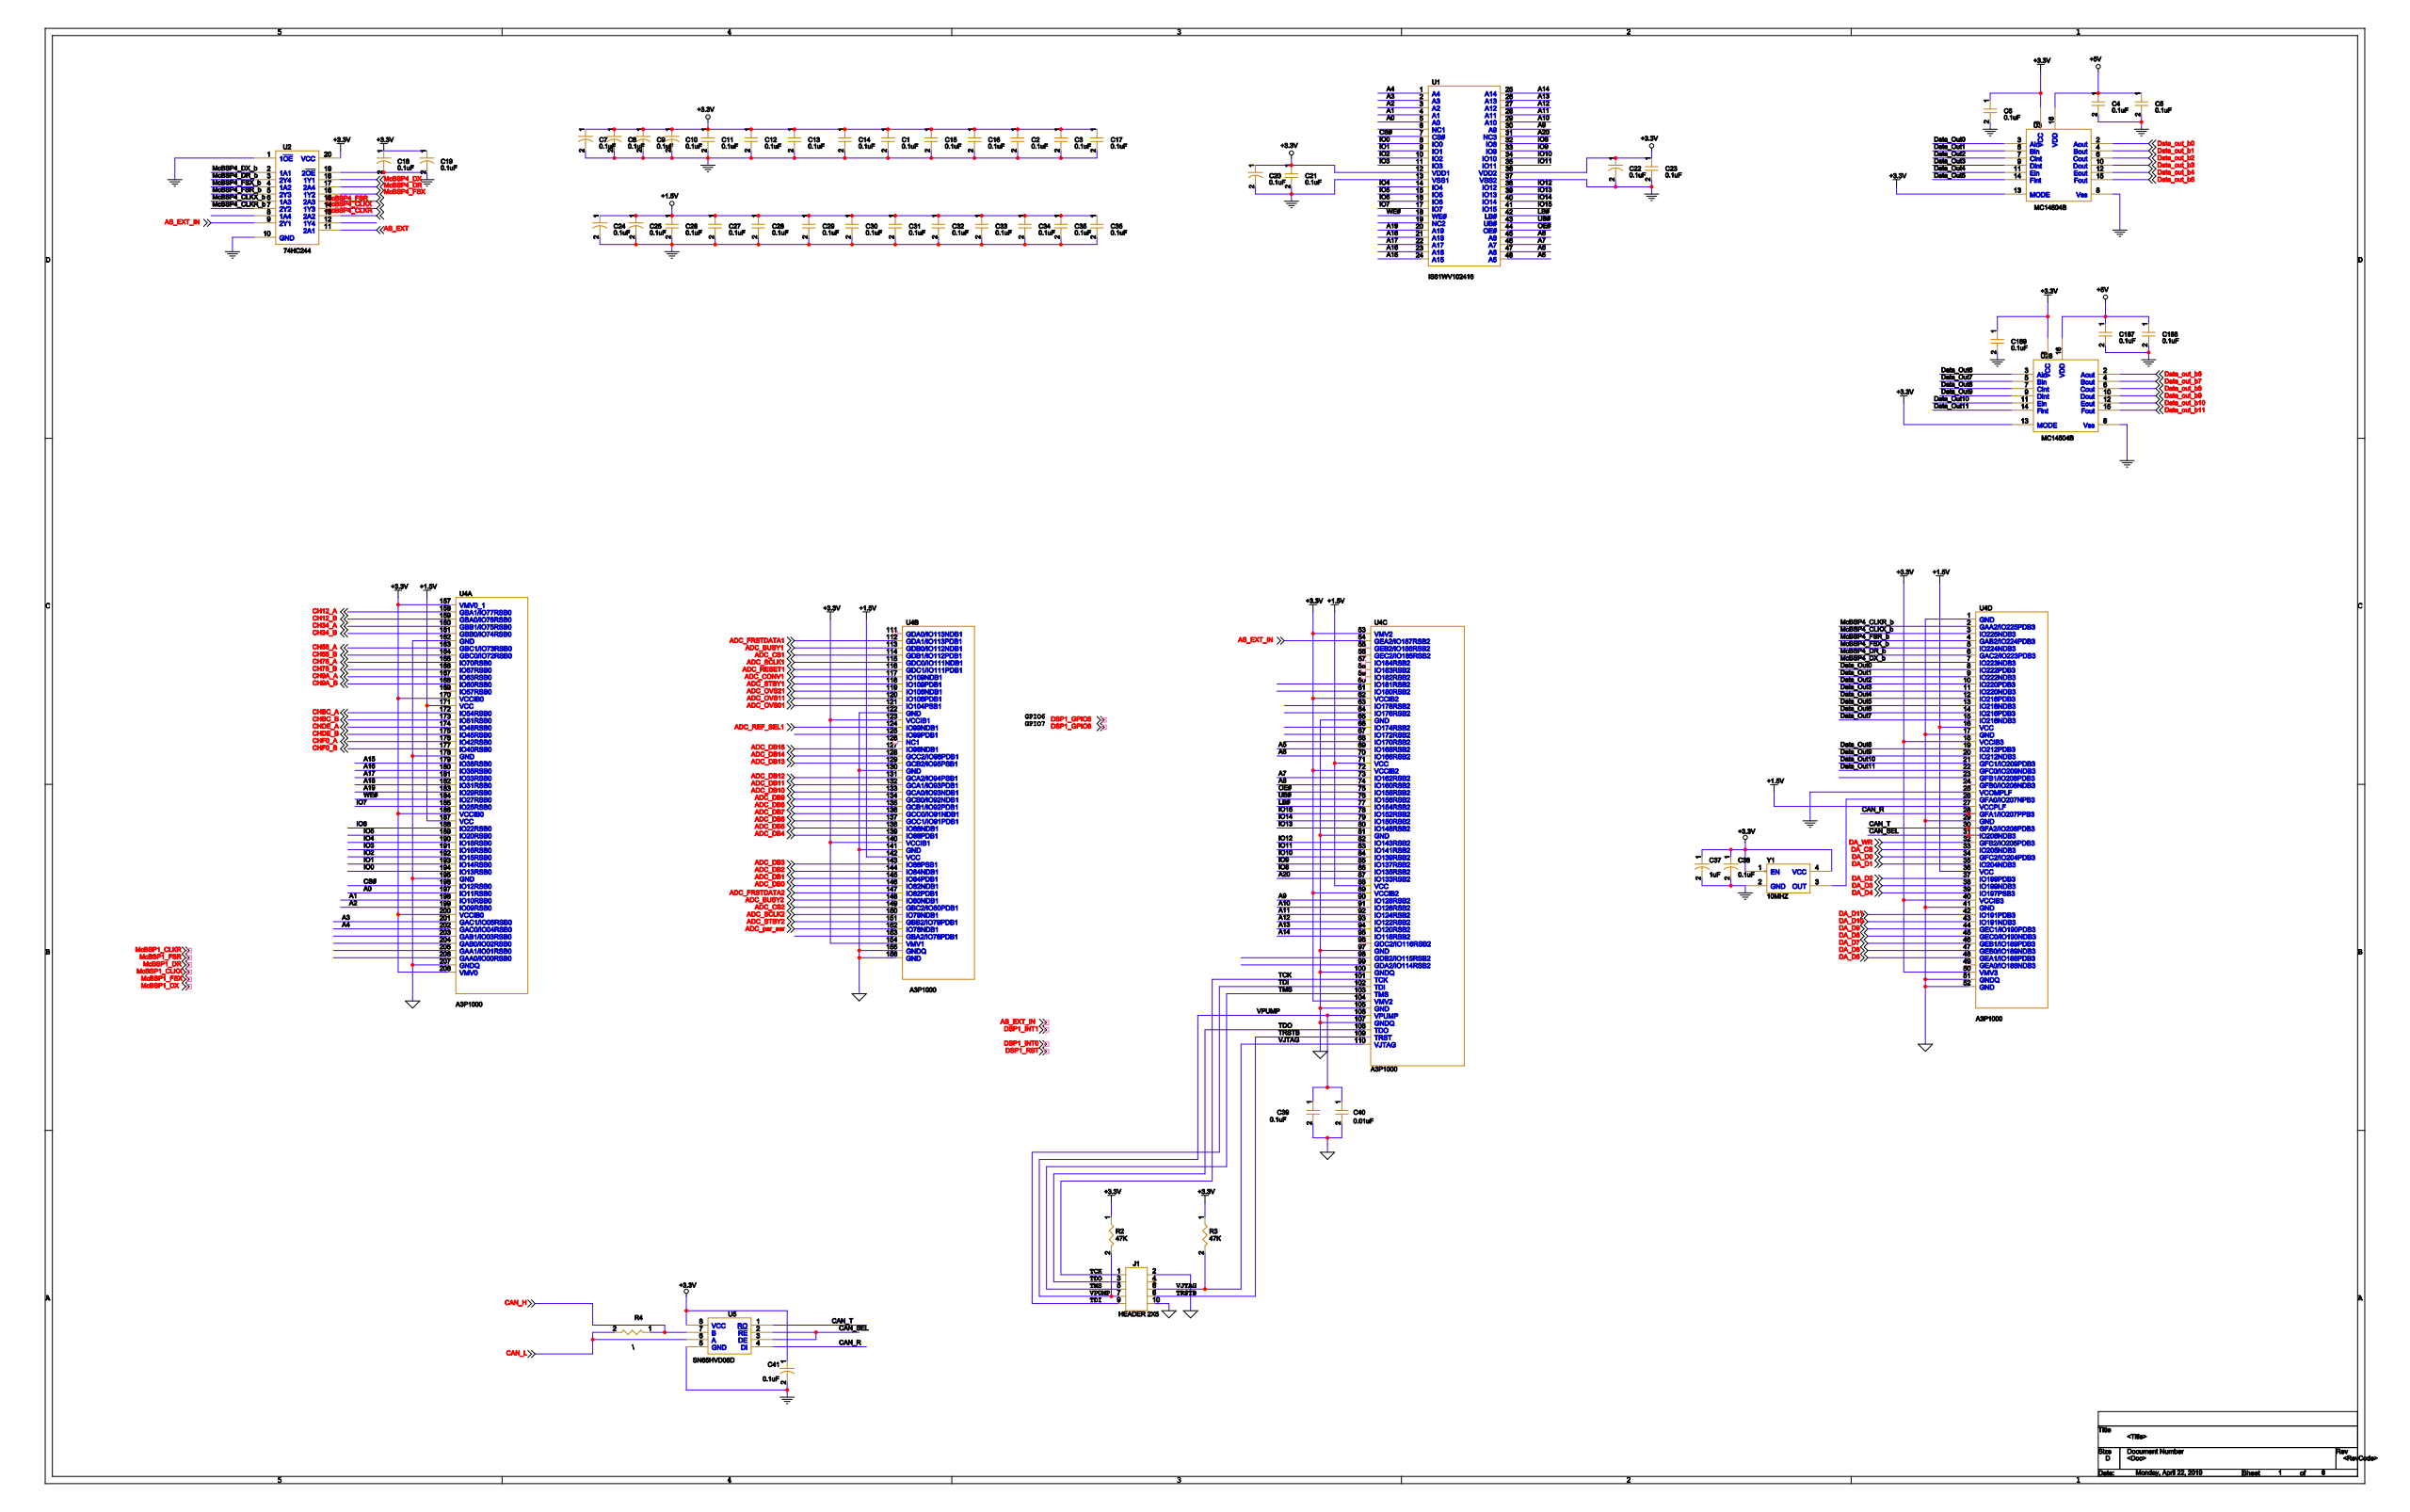Circuit board | Cadence Allegro | 362 parts | 391 nets | one sheet of the schematic
Parts on this sheet (reference | value | footprint):
C1 | 0.1uF | 1206
C2 | 0.1uF | 1206
C3 | 0.1uF | 1206
C4 | 0.1uF | 1206
C5 | 0.1uF | 1206
C6 | 0.1uF | 1206
C7 | 0.1uF | 1206
C8 | 0.1uF | 1206
C9 | 0.1uF | 1206
C10 | 0.1uF | 1206
C11 | 0.1uF | 1206
C12 | 0.1uF | 1206
C13 | 0.1uF | 1206
C14 | 0.1uF | 1206
C15 | 0.1uF | 1206
C16 | 0.1uF | 1206
C17 | 0.1uF | 1206
C18 | 0.1uF | 1206
C19 | 0.1uF | 1206
C20 | 0.1uF | 1206
C21 | 0.1uF | 1206
C22 | 0.1uF | 1206
C23 | 0.1uF | 1206
C24 | 0.1uF | 1206
C25 | 0.1uF | 1206
C26 | 0.1uF | 1206
C27 | 0.1uF | 1206
C28 | 0.1uF | 1206
C29 | 0.1uF | 1206
C30 | 0.1uF | 1206
C31 | 0.1uF | 1206
C32 | 0.1uF | 1206
C33 | 0.1uF | 1206
C34 | 0.1uF | 1206
C35 | 0.1uF | 1206
C36 | 0.1uF | 1206
C37 | 1uF | 1206
C38 | 0.1uF | 1206
C39 | 0.1uF | 1206
C40 | 0.01uF | 1206
C41 | 0.1uF | 1206
C187 | 0.1uF | 1206
C188 | 0.1uF | 1206
C189 | 0.1uF | 1206
J1 | HEADER 2X5 | HDR5X2_6240_ST
R2 | 47K | 0805
R3 | 47K | 0805
R4 | \ | 1206
U1 | IS61WV102416 | TSSOP48W
U2 | 74HC244 | SOIC20
U3 | MC14504B | SOIC16
U4 | A3P1000 | PQFP208
U5 | SN65HVD08D | SO-8
U28 | MC14504B | SOIC16
Y1 | 10MHZ | OSC-5X7MM
Nets of these parts (net: part-pin ...):
A0: U1-5 U4-197
A1: U1-4 U4-198
A10: U1-29 U4-91
A11: U1-28 U4-92
A12: U1-27 U4-93
A13: U1-26 U4-94
A14: U1-25 U4-95
A15: U1-24 U4-179
A16: U1-23 U4-180
A17: U1-22 U4-181
A18: U1-21 U4-182
A19: U1-20 U4-183
A2: U1-3 U4-199
A3: U1-2 U4-201
A4: U1-1 U4-202
A5: U1-48 U4-69
A6: U1-47 U4-70
A7: U1-46 U4-73
A8: U1-45 U4-74
A9: U1-30 U4-90
CS#: U1-7 U4-196
IO0: U1-8 U4-194
IO1: U1-9 U4-193
IO10: U1-34 U4-84
IO11: U1-35 U4-83
IO12: U1-38 U4-82
IO13: U1-39 U4-80
IO14: U1-40 U4-79
IO15: U1-41 U4-78
IO2: U1-10 U4-192
IO3: U1-11 U4-191
IO4: U1-14 U4-190
IO5: U1-15 U4-189
IO6: U1-16 U4-188
IO7: U1-17 U4-185
IO8: U1-32 U4-86
IO9: U1-33 U4-85
LB#: U1-42 U4-77
A20: U1-31 U4-87
OE#: U1-44 U4-75
UB#: U1-43 U4-76
+3.3V: C1-1 C2-1 C3-1 C6-1 C7-1 C8-1 C9-1 C10-1 C11-1 C12-1 C13-1 C14-1 C15-1 C16-1 C17-1 C18-1 C19-1 C20-1 C21-1 C22-1 C23-1 C37-1 C38-1 C41-1 C189-1 R2-1 R3-1 U2-20 U3-1 U3-13 U5-8 U28-1 U28-13 Y1-1 Y1-4 U1-12 U1-36 U4-18 U4-40 U4-50 U4-53 U4-62 U4-72 U4-89 U4-104 U4-123 U4-140 U4-154 U4-157 U4-170 U4-186 U4-200 U4-208
DGND: C1-2 C2-2 C3-2 C4-2 C5-2 C6-2 C7-2 C8-2 C9-2 C10-2 C11-2 C12-2 C13-2 C14-2 C15-2 C16-2 C17-2 C18-2 C19-2 C20-2 C21-2 C22-2 C23-2 C24-2 C25-2 C26-2 C27-2 C28-2 C29-2 C30-2 C31-2 C32-2 C33-2 C34-2 C35-2 C36-2 C37-2 C38-2 C39-2 C40-2 C41-2 C187-2 C188-2 C189-2 J1-2 J1-10 U2-1 U2-10 U2-19 U3-8 U5-5 U28-8 Y1-2 U1-13 U1-37 U4-1 U4-17 U4-25 U4-29 U4-41 U4-51 U4-52 U4-65 U4-81 U4-97 U4-100 U4-105 U4-107 U4-122 U4-130 U4-141 U4-155 U4-156 U4-162 U4-178 U4-195 U4-207
WE#: U1-18 U4-184
DA_CS: U4-33
DA_D0: U4-34
DA_D1: U4-35
DA_D10: U4-43
DA_D11: U4-42
DA_D2: U4-37
DA_D3: U4-38
DA_D4: U4-39
DA_D5: U4-48
DA_D6: U4-47
DA_D7: U4-46
DA_D8: U4-45
DA_D9: U4-44
+5.0V: C4-1 C5-1 C187-1 C188-1 U3-16 U28-16
DA_WR: U4-32
ADC_BUSY2: U4-148
ADC_CONV1: U4-117
ADC_DB0: U4-146
ADC_DB1: U4-145
ADC_DB10: U4-133
ADC_DB11: U4-132
ADC_DB12: U4-131
ADC_DB13: U4-129
ADC_DB14: U4-128
ADC_DB15: U4-127
ADC_DB2: U4-144
ADC_DB3: U4-143
ADC_DB4: U4-139
ADC_DB5: U4-138
ADC_DB6: U4-137
ADC_DB7: U4-136
ADC_DB8: U4-135
ADC_DB9: U4-134
ADC_FRSTDATA2: U4-147
ADC_OVS01: U4-121
ADC_OVS11: U4-120
ADC_OVS21: U4-119
ADC_REF_SEL1: U4-124
ADC_RESET1: U4-116
ADC_STBY2: U4-151
ADC_CS2: U4-149
ADC_SCLK2: U4-150
ADC_BUSY1: U4-113
ADC_FRSTDATA1: U4-112
ADC_STBY1: U4-118
ADC_CS1: U4-114
ADC_SCLK1: U4-115
MCBSP4_DX_B: U2-2 U4-7
MCBSP4_FSX_B: U2-4 U4-5
MCBSP4_CLKX_B: U2-6 U4-3
N17245333: U2-8
MCBSP4_DX: U2-18
MCBSP4_FSX: U2-16
MCBSP4_CLKX: U2-14
N17245355: U2-12
AS_EXT: U2-11
MCBSP4_CLKR: U2-13
MCBSP4_FSR: U2-15
MCBSP4_DR: U2-17
AS_EXT_IN: U2-9 U4-54
MCBSP4_CLKR_B: U2-7 U4-2
MCBSP4_FSR_B: U2-5 U4-4
MCBSP4_DR_B: U2-3 U4-6
DATA_OUT6: U28-3 U4-14
DATA_OUT_B6: U28-2
DATA_OUT7: U28-5 U4-15
DATA_OUT_B7: U28-4
DATA_OUT8: U28-7 U4-19
DATA_OUT_B8: U28-6
DATA_OUT9: U28-9 U4-20
DATA_OUT_B9: U28-10
DATA_OUT10: U28-11 U4-21
DATA_OUT_B10: U28-12
DATA_OUT11: U28-14 U4-22
DATA_OUT_B11: U28-15
DATA_OUT0: U3-3 U4-8
DATA_OUT_B0: U3-2
DATA_OUT1: U3-5 U4-9
DATA_OUT_B1: U3-4
DATA_OUT2: U3-7 U4-10
DATA_OUT_B2: U3-6
DATA_OUT3: U3-9 U4-11
DATA_OUT_B3: U3-10
DATA_OUT4: U3-11 U4-12
DATA_OUT_B4: U3-12
DATA_OUT5: U3-14 U4-13
DATA_OUT_B5: U3-15
CHF0_A: U4-176
CHF0_B: U4-177
CH78_A: U4-165
CH78_B: U4-166
CHDE_A: U4-174
CHDE_B: U4-175
CH56_A: U4-163
CH56_B: U4-164
CHBC_A: U4-172
CHBC_B: U4-173
CH34_A: U4-160
CH34_B: U4-161
CH9A_A: U4-167
CH9A_B: U4-168
CH12_A: U4-158
CH12_B: U4-159
CAN_L: R4-2 U5-6
CAN_H: R4-1 U5-7
CAN_SEL: U5-2 U5-3 U4-31
CAN_R: U5-4 U4-28
CAN_T: U5-1 U4-30
+1.5V: C24-1 C25-1 C26-1 C27-1 C28-1 C29-1 C30-1 C31-1 C32-1 C33-1 C34-1 C35-1 C36-1 U4-16 U4-27 U4-36 U4-71 U4-88 U4-142 U4-171 U4-187
TCK: J1-1 U4-101
TDI: J1-9 U4-102
TDO: J1-3 U4-108
TMS: J1-5 U4-103
TRSTB: J1-8 U4-109
VJTAG: J1-6 R3-2 U4-110
VPUMP: C39-1 C40-1 J1-7 R2-2 U4-106
N17245537: Y1-3 U4-26